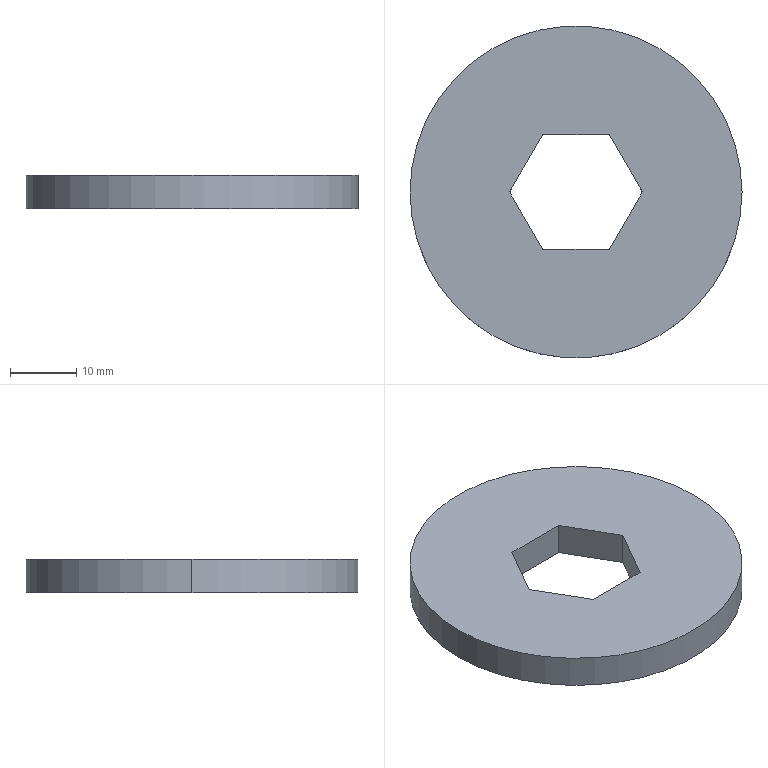Part | NX | 1 solid | 10 faces | box 50 x 50 x 5 mm | volume 8518 mm3 | plane 8 | cylinder 2 | commonest cylinder face diameters 50 x2
STEP:
#1=CARTESIAN_POINT('',(25.,0.,5.));
#2=VERTEX_POINT('',#1);
#3=CARTESIAN_POINT('',(-25.,0.,5.));
#4=VERTEX_POINT('',#3);
#5=CARTESIAN_POINT('',(0.,0.,5.));
#6=DIRECTION('',(0.,0.,1.));
#7=DIRECTION('',(1.,0.,0.));
#8=AXIS2_PLACEMENT_3D('',#5,#6,#7);
#9=CIRCLE('',#8,25.);
#10=EDGE_CURVE('',#2,#4,#9,.T.);
#11=ORIENTED_EDGE('',*,*,#10,.F.);
#12=CARTESIAN_POINT('',(25.,0.,0.));
#13=VERTEX_POINT('',#12);
#14=CARTESIAN_POINT('',(25.,0.,5.));
#15=DIRECTION('',(0.,0.,1.));
#16=VECTOR('',#15,1.);
#17=LINE('',#14,#16);
#18=EDGE_CURVE('',#13,#2,#17,.T.);
#19=ORIENTED_EDGE('',*,*,#18,.F.);
#20=CARTESIAN_POINT('',(-25.,0.,0.));
#21=VERTEX_POINT('',#20);
#22=CARTESIAN_POINT('',(0.,0.,0.));
#23=DIRECTION('',(0.,0.,1.));
#24=DIRECTION('',(1.,0.,0.));
#25=AXIS2_PLACEMENT_3D('',#22,#23,#24);
#26=CIRCLE('',#25,25.);
#27=EDGE_CURVE('',#13,#21,#26,.T.);
#28=ORIENTED_EDGE('',*,*,#27,.T.);
#29=CARTESIAN_POINT('',(-25.,0.,5.));
#30=DIRECTION('',(0.,0.,1.));
#31=VECTOR('',#30,1.);
#32=LINE('',#29,#31);
#33=EDGE_CURVE('',#21,#4,#32,.T.);
#34=ORIENTED_EDGE('',*,*,#33,.T.);
#35=EDGE_LOOP('',(#11,#19,#28,#34));
#36=FACE_OUTER_BOUND('',#35,.T.);
#37=CARTESIAN_POINT('',(0.,0.,5.));
#38=DIRECTION('',(0.,0.,-1.));
#39=DIRECTION('',(-1.,0.,0.));
#40=AXIS2_PLACEMENT_3D('',#37,#38,#39);
#41=CYLINDRICAL_SURFACE('',#40,25.);
#42=ADVANCED_FACE('',(#36),#41,.T.);
#43=CARTESIAN_POINT('',(0.,0.,5.));
#44=DIRECTION('',(0.,0.,1.));
#45=DIRECTION('',(1.,0.,0.));
#46=AXIS2_PLACEMENT_3D('',#43,#44,#45);
#47=CIRCLE('',#46,25.);
#48=EDGE_CURVE('',#4,#2,#47,.T.);
#49=ORIENTED_EDGE('',*,*,#48,.T.);
#50=ORIENTED_EDGE('',*,*,#10,.T.);
#51=EDGE_LOOP('',(#49,#50));
#52=FACE_BOUND('',#51,.T.);
#53=CARTESIAN_POINT('',(10.,0.,5.));
#54=VERTEX_POINT('',#53);
#55=CARTESIAN_POINT('',(5.,8.66,5.));
#56=VERTEX_POINT('',#55);
#57=CARTESIAN_POINT('',(10.,0.,5.));
#58=DIRECTION('',(-0.5,0.866,0.));
#59=VECTOR('',#58,1.);
#60=LINE('',#57,#59);
#61=EDGE_CURVE('',#54,#56,#60,.T.);
#62=ORIENTED_EDGE('',*,*,#61,.F.);
#63=CARTESIAN_POINT('',(5.,-8.66,5.));
#64=VERTEX_POINT('',#63);
#65=CARTESIAN_POINT('',(5.,-8.66,5.));
#66=DIRECTION('',(0.5,0.866,0.));
#67=VECTOR('',#66,1.);
#68=LINE('',#65,#67);
#69=EDGE_CURVE('',#64,#54,#68,.T.);
#70=ORIENTED_EDGE('',*,*,#69,.F.);
#71=CARTESIAN_POINT('',(-5.,-8.66,5.));
#72=VERTEX_POINT('',#71);
#73=CARTESIAN_POINT('',(-5.,-8.66,5.));
#74=DIRECTION('',(1.,0.,0.));
#75=VECTOR('',#74,1.);
#76=LINE('',#73,#75);
#77=EDGE_CURVE('',#72,#64,#76,.T.);
#78=ORIENTED_EDGE('',*,*,#77,.F.);
#79=CARTESIAN_POINT('',(-10.,0.,5.));
#80=VERTEX_POINT('',#79);
#81=CARTESIAN_POINT('',(-10.,0.,5.));
#82=DIRECTION('',(0.5,-0.866,0.));
#83=VECTOR('',#82,1.);
#84=LINE('',#81,#83);
#85=EDGE_CURVE('',#80,#72,#84,.T.);
#86=ORIENTED_EDGE('',*,*,#85,.F.);
#87=CARTESIAN_POINT('',(-5.,8.66,5.));
#88=VERTEX_POINT('',#87);
#89=CARTESIAN_POINT('',(-5.,8.66,5.));
#90=DIRECTION('',(-0.5,-0.866,0.));
#91=VECTOR('',#90,1.);
#92=LINE('',#89,#91);
#93=EDGE_CURVE('',#88,#80,#92,.T.);
#94=ORIENTED_EDGE('',*,*,#93,.F.);
#95=CARTESIAN_POINT('',(5.,8.66,5.));
#96=DIRECTION('',(-1.,0.,0.));
#97=VECTOR('',#96,1.);
#98=LINE('',#95,#97);
#99=EDGE_CURVE('',#56,#88,#98,.T.);
#100=ORIENTED_EDGE('',*,*,#99,.F.);
#101=EDGE_LOOP('',(#62,#70,#78,#86,#94,#100));
#102=FACE_BOUND('',#101,.T.);
#103=CARTESIAN_POINT('',(0.,0.,5.));
#104=DIRECTION('',(0.,0.,1.));
#105=DIRECTION('',(1.,0.,0.));
#106=AXIS2_PLACEMENT_3D('',#103,#104,#105);
#107=PLANE('',#106);
#108=ADVANCED_FACE('',(#52,#102),#107,.T.);
#109=CARTESIAN_POINT('',(0.,0.,0.));
#110=DIRECTION('',(0.,0.,1.));
#111=DIRECTION('',(1.,0.,0.));
#112=AXIS2_PLACEMENT_3D('',#109,#110,#111);
#113=CIRCLE('',#112,25.);
#114=EDGE_CURVE('',#21,#13,#113,.T.);
#115=ORIENTED_EDGE('',*,*,#114,.F.);
#116=ORIENTED_EDGE('',*,*,#27,.F.);
#117=EDGE_LOOP('',(#115,#116));
#118=FACE_BOUND('',#117,.T.);
#119=CARTESIAN_POINT('',(5.,-8.66,0.));
#120=VERTEX_POINT('',#119);
#121=CARTESIAN_POINT('',(10.,0.,0.));
#122=VERTEX_POINT('',#121);
#123=CARTESIAN_POINT('',(5.,-8.66,0.));
#124=DIRECTION('',(0.5,0.866,0.));
#125=VECTOR('',#124,1.);
#126=LINE('',#123,#125);
#127=EDGE_CURVE('',#120,#122,#126,.T.);
#128=ORIENTED_EDGE('',*,*,#127,.T.);
#129=CARTESIAN_POINT('',(5.,8.66,0.));
#130=VERTEX_POINT('',#129);
#131=CARTESIAN_POINT('',(10.,0.,0.));
#132=DIRECTION('',(-0.5,0.866,0.));
#133=VECTOR('',#132,1.);
#134=LINE('',#131,#133);
#135=EDGE_CURVE('',#122,#130,#134,.T.);
#136=ORIENTED_EDGE('',*,*,#135,.T.);
#137=CARTESIAN_POINT('',(-5.,8.66,0.));
#138=VERTEX_POINT('',#137);
#139=CARTESIAN_POINT('',(5.,8.66,0.));
#140=DIRECTION('',(-1.,0.,0.));
#141=VECTOR('',#140,1.);
#142=LINE('',#139,#141);
#143=EDGE_CURVE('',#130,#138,#142,.T.);
#144=ORIENTED_EDGE('',*,*,#143,.T.);
#145=CARTESIAN_POINT('',(-10.,0.,0.));
#146=VERTEX_POINT('',#145);
#147=CARTESIAN_POINT('',(-5.,8.66,0.));
#148=DIRECTION('',(-0.5,-0.866,0.));
#149=VECTOR('',#148,1.);
#150=LINE('',#147,#149);
#151=EDGE_CURVE('',#138,#146,#150,.T.);
#152=ORIENTED_EDGE('',*,*,#151,.T.);
#153=CARTESIAN_POINT('',(-5.,-8.66,0.));
#154=VERTEX_POINT('',#153);
#155=CARTESIAN_POINT('',(-10.,0.,0.));
#156=DIRECTION('',(0.5,-0.866,0.));
#157=VECTOR('',#156,1.);
#158=LINE('',#155,#157);
#159=EDGE_CURVE('',#146,#154,#158,.T.);
#160=ORIENTED_EDGE('',*,*,#159,.T.);
#161=CARTESIAN_POINT('',(-5.,-8.66,0.));
#162=DIRECTION('',(1.,0.,0.));
#163=VECTOR('',#162,1.);
#164=LINE('',#161,#163);
#165=EDGE_CURVE('',#154,#120,#164,.T.);
#166=ORIENTED_EDGE('',*,*,#165,.T.);
#167=EDGE_LOOP('',(#128,#136,#144,#152,#160,#166));
#168=FACE_BOUND('',#167,.T.);
#169=CARTESIAN_POINT('',(0.,0.,0.));
#170=DIRECTION('',(0.,0.,1.));
#171=DIRECTION('',(1.,0.,0.));
#172=AXIS2_PLACEMENT_3D('',#169,#170,#171);
#173=PLANE('',#172);
#174=ADVANCED_FACE('',(#118,#168),#173,.F.);
#175=ORIENTED_EDGE('',*,*,#18,.T.);
#176=ORIENTED_EDGE('',*,*,#48,.F.);
#177=ORIENTED_EDGE('',*,*,#33,.F.);
#178=ORIENTED_EDGE('',*,*,#114,.T.);
#179=EDGE_LOOP('',(#175,#176,#177,#178));
#180=FACE_OUTER_BOUND('',#179,.T.);
#181=CARTESIAN_POINT('',(0.,0.,5.));
#182=DIRECTION('',(0.,0.,-1.));
#183=DIRECTION('',(-1.,0.,0.));
#184=AXIS2_PLACEMENT_3D('',#181,#182,#183);
#185=CYLINDRICAL_SURFACE('',#184,25.);
#186=ADVANCED_FACE('',(#180),#185,.T.);
#187=ORIENTED_EDGE('',*,*,#127,.F.);
#188=CARTESIAN_POINT('',(5.,-8.66,5.));
#189=DIRECTION('',(0.,0.,-1.));
#190=VECTOR('',#189,1.);
#191=LINE('',#188,#190);
#192=EDGE_CURVE('',#64,#120,#191,.T.);
#193=ORIENTED_EDGE('',*,*,#192,.F.);
#194=ORIENTED_EDGE('',*,*,#69,.T.);
#195=CARTESIAN_POINT('',(10.,0.,5.));
#196=DIRECTION('',(0.,0.,-1.));
#197=VECTOR('',#196,1.);
#198=LINE('',#195,#197);
#199=EDGE_CURVE('',#54,#122,#198,.T.);
#200=ORIENTED_EDGE('',*,*,#199,.T.);
#201=EDGE_LOOP('',(#187,#193,#194,#200));
#202=FACE_OUTER_BOUND('',#201,.T.);
#203=CARTESIAN_POINT('',(5.,-8.66,5.));
#204=DIRECTION('',(-0.866,0.5,0.));
#205=DIRECTION('',(-0.5,-0.866,0.));
#206=AXIS2_PLACEMENT_3D('',#203,#204,#205);
#207=PLANE('',#206);
#208=ADVANCED_FACE('',(#202),#207,.T.);
#209=ORIENTED_EDGE('',*,*,#135,.F.);
#210=ORIENTED_EDGE('',*,*,#199,.F.);
#211=ORIENTED_EDGE('',*,*,#61,.T.);
#212=CARTESIAN_POINT('',(5.,8.66,5.));
#213=DIRECTION('',(0.,0.,-1.));
#214=VECTOR('',#213,1.);
#215=LINE('',#212,#214);
#216=EDGE_CURVE('',#56,#130,#215,.T.);
#217=ORIENTED_EDGE('',*,*,#216,.T.);
#218=EDGE_LOOP('',(#209,#210,#211,#217));
#219=FACE_OUTER_BOUND('',#218,.T.);
#220=CARTESIAN_POINT('',(10.,0.,5.));
#221=DIRECTION('',(-0.866,-0.5,0.));
#222=DIRECTION('',(0.5,-0.866,0.));
#223=AXIS2_PLACEMENT_3D('',#220,#221,#222);
#224=PLANE('',#223);
#225=ADVANCED_FACE('',(#219),#224,.T.);
#226=ORIENTED_EDGE('',*,*,#143,.F.);
#227=ORIENTED_EDGE('',*,*,#216,.F.);
#228=ORIENTED_EDGE('',*,*,#99,.T.);
#229=CARTESIAN_POINT('',(-5.,8.66,5.));
#230=DIRECTION('',(0.,0.,-1.));
#231=VECTOR('',#230,1.);
#232=LINE('',#229,#231);
#233=EDGE_CURVE('',#88,#138,#232,.T.);
#234=ORIENTED_EDGE('',*,*,#233,.T.);
#235=EDGE_LOOP('',(#226,#227,#228,#234));
#236=FACE_OUTER_BOUND('',#235,.T.);
#237=CARTESIAN_POINT('',(5.,8.66,5.));
#238=DIRECTION('',(0.,-1.,0.));
#239=DIRECTION('',(1.,0.,0.));
#240=AXIS2_PLACEMENT_3D('',#237,#238,#239);
#241=PLANE('',#240);
#242=ADVANCED_FACE('',(#236),#241,.T.);
#243=ORIENTED_EDGE('',*,*,#151,.F.);
#244=ORIENTED_EDGE('',*,*,#233,.F.);
#245=ORIENTED_EDGE('',*,*,#93,.T.);
#246=CARTESIAN_POINT('',(-10.,0.,5.));
#247=DIRECTION('',(0.,0.,-1.));
#248=VECTOR('',#247,1.);
#249=LINE('',#246,#248);
#250=EDGE_CURVE('',#80,#146,#249,.T.);
#251=ORIENTED_EDGE('',*,*,#250,.T.);
#252=EDGE_LOOP('',(#243,#244,#245,#251));
#253=FACE_OUTER_BOUND('',#252,.T.);
#254=CARTESIAN_POINT('',(-5.,8.66,5.));
#255=DIRECTION('',(0.866,-0.5,0.));
#256=DIRECTION('',(0.5,0.866,0.));
#257=AXIS2_PLACEMENT_3D('',#254,#255,#256);
#258=PLANE('',#257);
#259=ADVANCED_FACE('',(#253),#258,.T.);
#260=ORIENTED_EDGE('',*,*,#159,.F.);
#261=ORIENTED_EDGE('',*,*,#250,.F.);
#262=ORIENTED_EDGE('',*,*,#85,.T.);
#263=CARTESIAN_POINT('',(-5.,-8.66,5.));
#264=DIRECTION('',(0.,0.,-1.));
#265=VECTOR('',#264,1.);
#266=LINE('',#263,#265);
#267=EDGE_CURVE('',#72,#154,#266,.T.);
#268=ORIENTED_EDGE('',*,*,#267,.T.);
#269=EDGE_LOOP('',(#260,#261,#262,#268));
#270=FACE_OUTER_BOUND('',#269,.T.);
#271=CARTESIAN_POINT('',(-10.,0.,5.));
#272=DIRECTION('',(0.866,0.5,0.));
#273=DIRECTION('',(-0.5,0.866,0.));
#274=AXIS2_PLACEMENT_3D('',#271,#272,#273);
#275=PLANE('',#274);
#276=ADVANCED_FACE('',(#270),#275,.T.);
#277=ORIENTED_EDGE('',*,*,#165,.F.);
#278=ORIENTED_EDGE('',*,*,#267,.F.);
#279=ORIENTED_EDGE('',*,*,#77,.T.);
#280=ORIENTED_EDGE('',*,*,#192,.T.);
#281=EDGE_LOOP('',(#277,#278,#279,#280));
#282=FACE_OUTER_BOUND('',#281,.T.);
#283=CARTESIAN_POINT('',(-5.,-8.66,5.));
#284=DIRECTION('',(0.,1.,0.));
#285=DIRECTION('',(-1.,0.,0.));
#286=AXIS2_PLACEMENT_3D('',#283,#284,#285);
#287=PLANE('',#286);
#288=ADVANCED_FACE('',(#282),#287,.T.);
#289=CLOSED_SHELL('',(#42,#108,#174,#186,#208,#225,#242,#259,#276,#288));
#290=MANIFOLD_SOLID_BREP('',#289);
#291=(LENGTH_UNIT()NAMED_UNIT(*)SI_UNIT(.MILLI.,.METRE.));
#292=UNCERTAINTY_MEASURE_WITH_UNIT(LENGTH_MEASURE(0.00002),#291,'','');
#293=(NAMED_UNIT(*)PLANE_ANGLE_UNIT()SI_UNIT($,.RADIAN.));
#294=PLANE_ANGLE_MEASURE_WITH_UNIT(PLANE_ANGLE_MEASURE(0.01745),#293);
#295=DIMENSIONAL_EXPONENTS(0.,0.,0.,0.,0.,0.,0.);
#296=(CONVERSION_BASED_UNIT('DEGREE',#294)NAMED_UNIT(#295)PLANE_ANGLE_UNIT());
#297=(NAMED_UNIT(*)SI_UNIT($,.STERADIAN.)SOLID_ANGLE_UNIT());
#298=(GEOMETRIC_REPRESENTATION_CONTEXT(3)GLOBAL_UNCERTAINTY_ASSIGNED_CONTEXT((#292))GLOBAL_UNIT_ASSIGNED_CONTEXT((#291,#296,#297))REPRESENTATION_CONTEXT('',''));
#299=ADVANCED_BREP_SHAPE_REPRESENTATION('',(#290),#298);